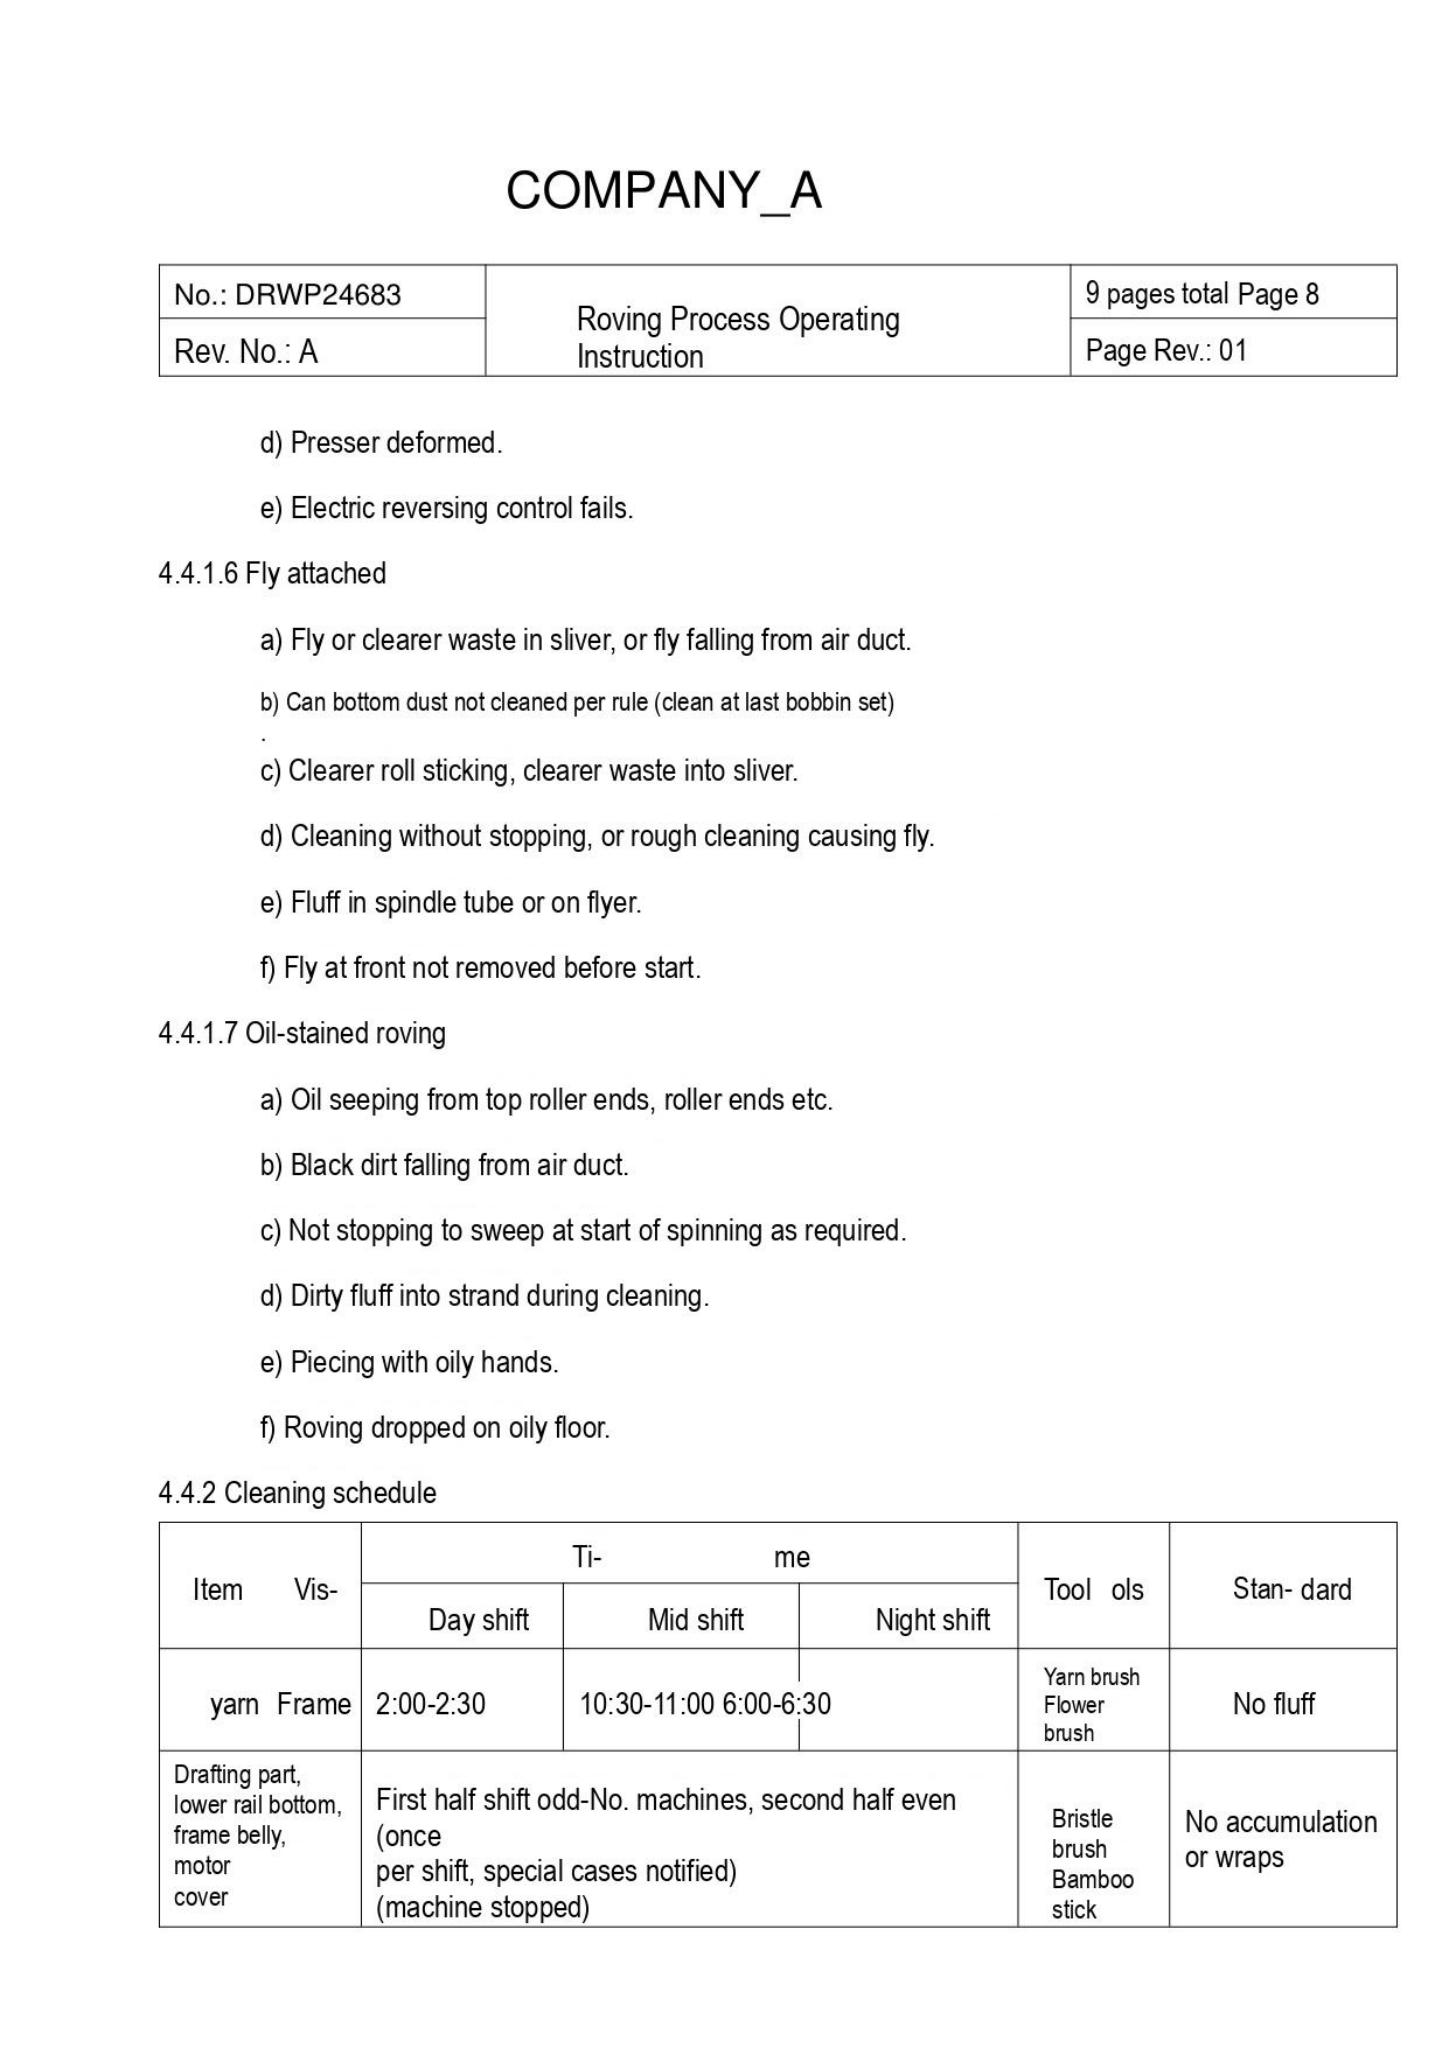COMPANY_A

| No.: DRWP24683 | Roving Process Operating Instruction | 9 pages total Page 8 |
|---|---|---|
| Rev. No.: A | | Page Rev.: 01 |

d) Presser deformed.

e) Electric reversing control fails.

4.4.1.6 Fly attached

a) Fly or clearer waste in sliver, or fly falling from air duct.

b) Can bottom dust not cleaned per rule (clean at last bobbin set)

.

c) Clearer roll sticking, clearer waste into sliver.

d) Cleaning without stopping, or rough cleaning causing fly.

e) Fluff in spindle tube or on flyer.

f) Fly at front not removed before start.

4.4.1.7 Oil-stained roving

a) Oil seeping from top roller ends, roller ends etc.

b) Black dirt falling from air duct.

c) Not stopping to sweep at start of spinning as required.

d) Dirty fluff into strand during cleaning.

e) Piecing with oily hands.

f) Roving dropped on oily floor.

4.4.2 Cleaning schedule

| Item Vis- | Ti- me | | | Tool ols | Stan- dard |
|---|---|---|---|---|---|
| | Day shift | Mid shift | Night shift | | |
| yarn Frame | 2:00-2:30 | 10:30-11:00 | 6:00-6:30 | Yarn brush Flower brush | No fluff |
| Drafting part, lower rail bottom, frame belly, motor cover | First half shift odd-No. machines, second half even (once per shift, special cases notified) (machine stopped) | | | Bristle brush Bamboo stick | No accumulation or wraps |
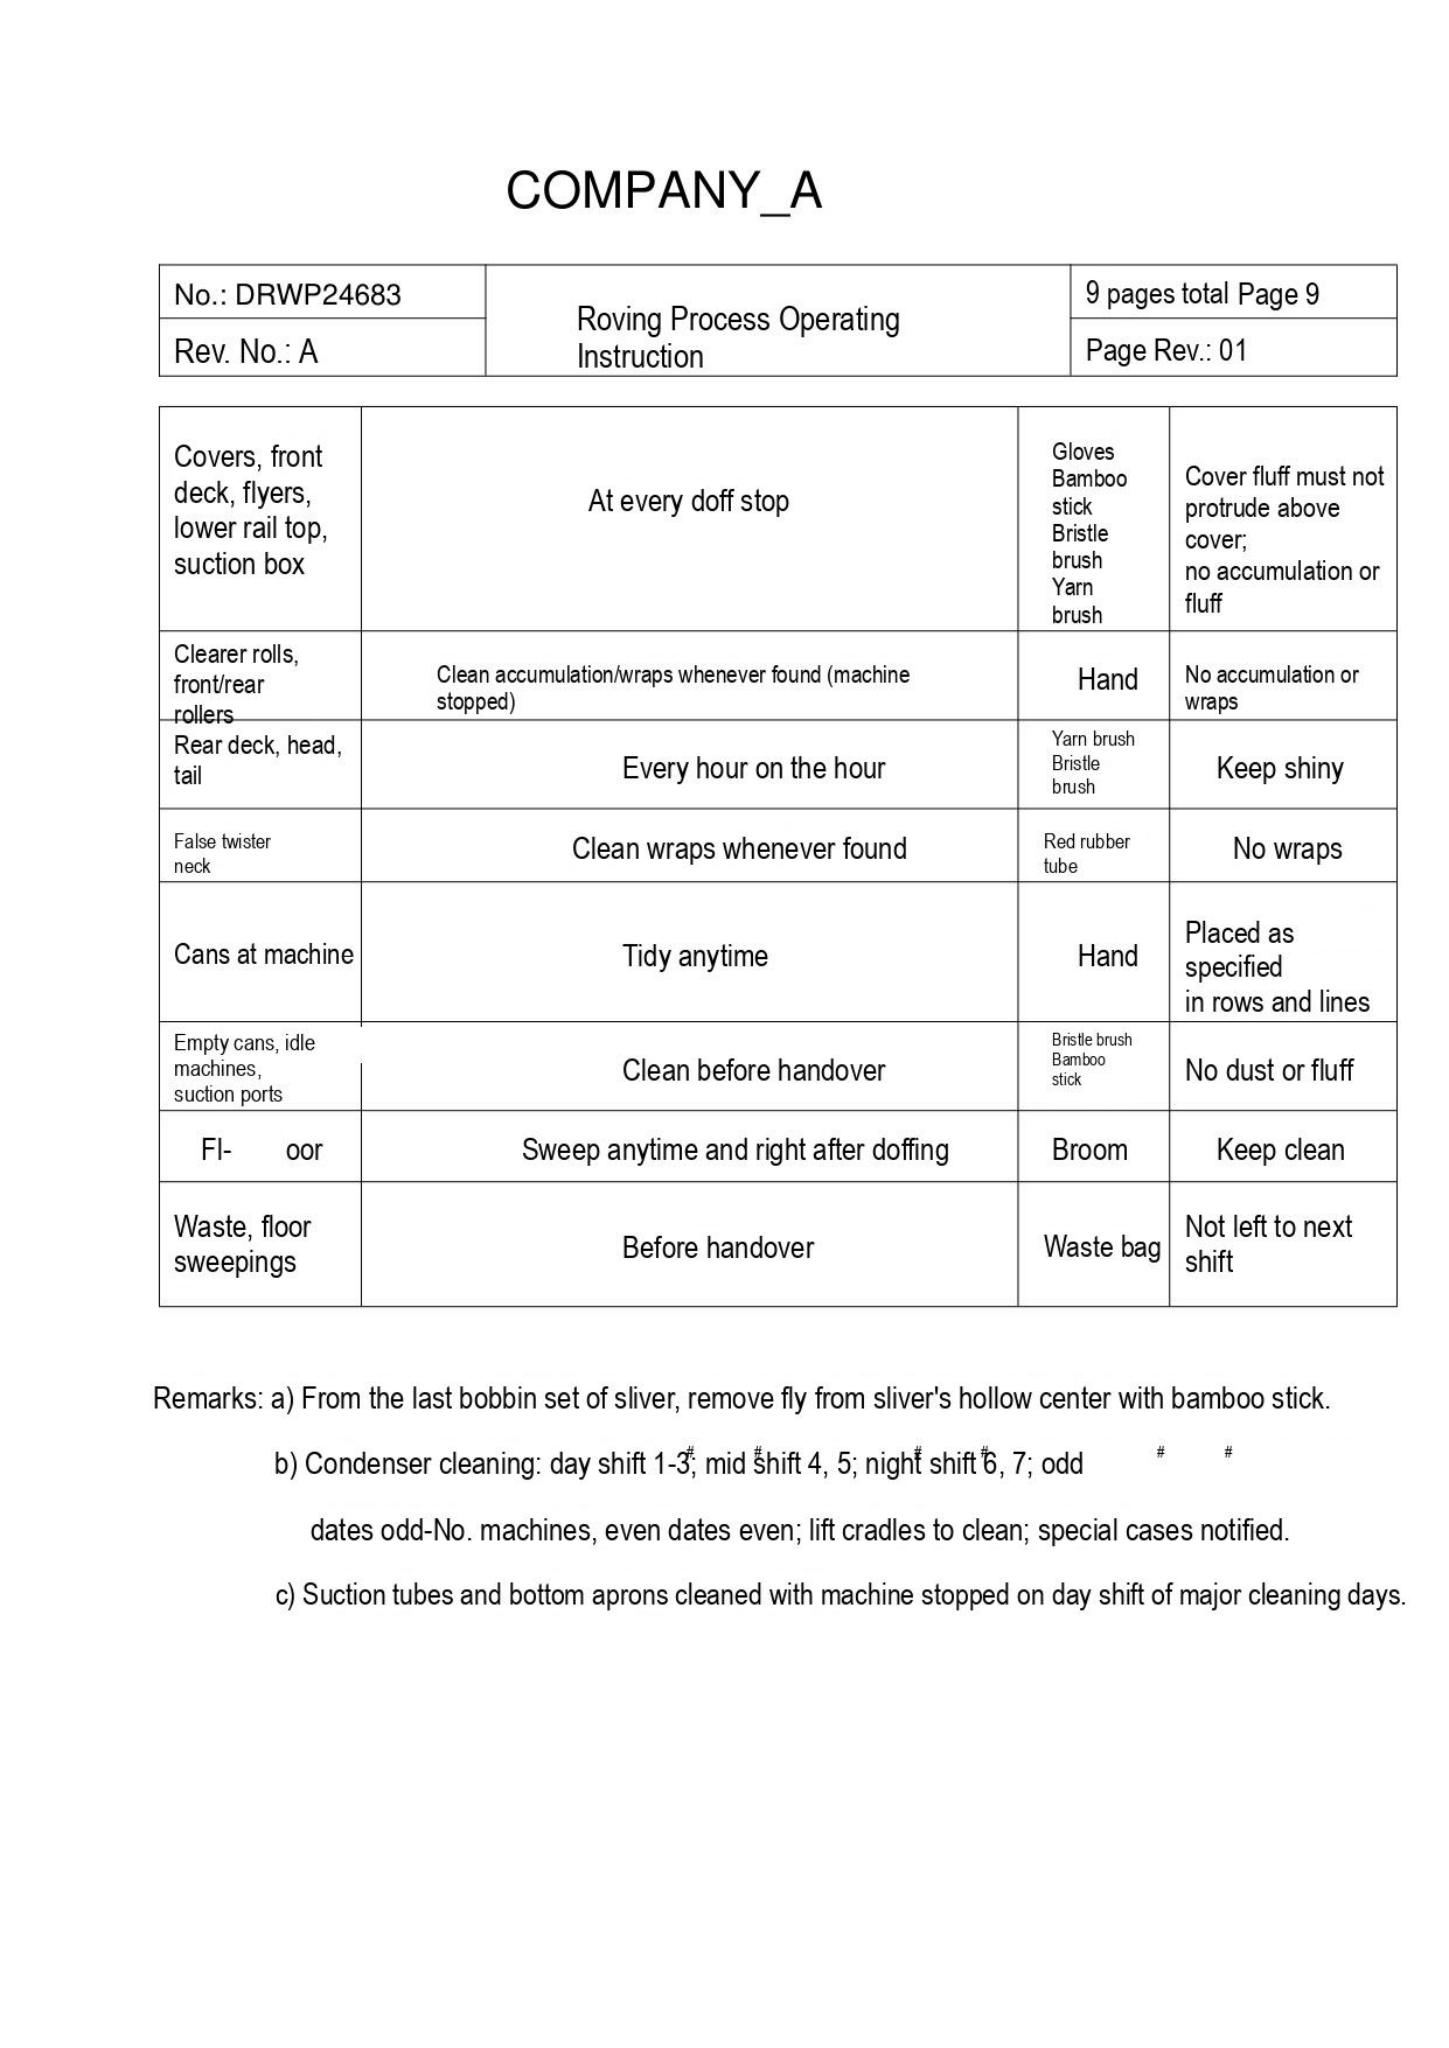COMPANY_A

| No.: DRWP24683 | Roving Process Operating Instruction | 9 pages total Page 9 |
|---|---|---|
| Rev. No.: A | | Page Rev.: 01 |

| | | | |
|---|---|---|---|
| Covers, front deck, flyers, lower rail top, suction box | At every doff stop | Gloves Bamboo stick Bristle brush Yarn brush | Cover fluff must not protrude above cover; no accumulation or fluff |
| Clearer rolls, front/rear rollers | Clean accumulation/wraps whenever found (machine stopped) | Hand | No accumulation or wraps |
| Rear deck, head, tail | Every hour on the hour | Yarn brush Bristle brush | Keep shiny |
| False twister neck | Clean wraps whenever found | Red rubber tube | No wraps |
| Cans at machine | Tidy anytime | Hand | Placed as specified in rows and lines |
| Empty cans, idle machines, suction ports | Clean before handover | Bristle brush Bamboo stick | No dust or fluff |
| Fl- oor | Sweep anytime and right after doffing | Broom | Keep clean |
| Waste, floor sweepings | Before handover | Waste bag | Not left to next shift |

Remarks: a) From the last bobbin set of sliver, remove fly from sliver's hollow center with bamboo stick.

b) Condenser cleaning: day shift 1-3#; mid shift 4#, 5#; night shift 6#, 7#; odd # #

dates odd-No. machines, even dates even; lift cradles to clean; special cases notified.

c) Suction tubes and bottom aprons cleaned with machine stopped on day shift of major cleaning days.